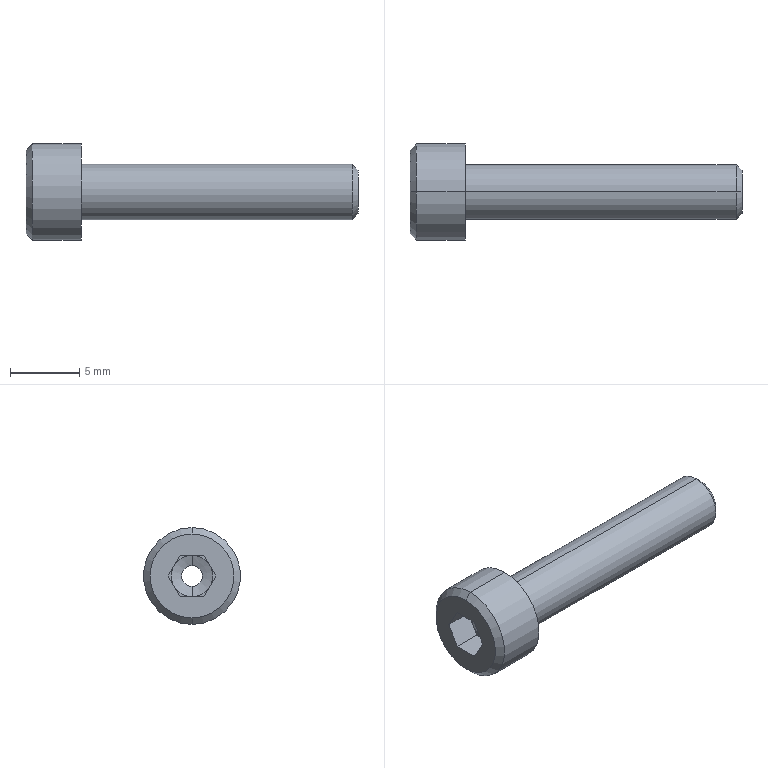Part | SolidWorks | features ICE 1, RevCut 1, Revolution 1 | 1 solid | 27 faces | box 24 x 7 x 7 mm | volume 346.79 mm3 | plane 15 | cylinder 6 | cone 6 | commonest cylinder face diameters 1.5 x2 4 x2 7 x2
STEP:
#1=CARTESIAN_POINT('',(20.,0.,-0.75));
#2=VERTEX_POINT('',#1);
#3=CARTESIAN_POINT('',(20.,0.,0.75));
#4=VERTEX_POINT('',#3);
#5=CARTESIAN_POINT('',(20.,0.,0.));
#6=DIRECTION('',(-1.,0.,0.));
#7=DIRECTION('',(0.,0.,1.));
#8=AXIS2_PLACEMENT_3D('',#5,#6,#7);
#9=CIRCLE('',#8,0.75);
#10=EDGE_CURVE('',#2,#4,#9,.T.);
#11=ORIENTED_EDGE('',*,*,#10,.F.);
#12=CARTESIAN_POINT('',(-1.727,0.,-0.75));
#13=VERTEX_POINT('',#12);
#14=CARTESIAN_POINT('',(20.,0.,-0.75));
#15=DIRECTION('',(-1.,0.,0.));
#16=VECTOR('',#15,1000.);
#17=LINE('',#14,#16);
#18=EDGE_CURVE('',#2,#13,#17,.T.);
#19=ORIENTED_EDGE('',*,*,#18,.T.);
#20=CARTESIAN_POINT('',(-1.727,0.,0.75));
#21=VERTEX_POINT('',#20);
#22=CARTESIAN_POINT('',(-1.727,0.,0.));
#23=DIRECTION('',(-1.,0.,0.));
#24=DIRECTION('',(0.,0.,1.));
#25=AXIS2_PLACEMENT_3D('',#22,#23,#24);
#26=CIRCLE('',#25,0.75);
#27=EDGE_CURVE('',#13,#21,#26,.T.);
#28=ORIENTED_EDGE('',*,*,#27,.T.);
#29=CARTESIAN_POINT('',(20.,0.,0.75));
#30=DIRECTION('',(-1.,0.,0.));
#31=VECTOR('',#30,1000.);
#32=LINE('',#29,#31);
#33=EDGE_CURVE('',#4,#21,#32,.T.);
#34=ORIENTED_EDGE('',*,*,#33,.F.);
#35=EDGE_LOOP('',(#11,#19,#28,#34));
#36=FACE_OUTER_BOUND('',#35,.T.);
#37=CARTESIAN_POINT('',(20.,0.,0.));
#38=DIRECTION('',(-1.,0.,0.));
#39=DIRECTION('',(0.,0.,1.));
#40=AXIS2_PLACEMENT_3D('',#37,#38,#39);
#41=CYLINDRICAL_SURFACE('',#40,0.75);
#42=ADVANCED_FACE('',(#36),#41,.F.);
#43=ORIENTED_EDGE('',*,*,#27,.F.);
#44=CARTESIAN_POINT('',(-2.,0.,-1.5));
#45=VERTEX_POINT('',#44);
#46=CARTESIAN_POINT('',(-1.727,0.,-0.75));
#47=DIRECTION('',(-0.342,0.,-0.9397));
#48=VECTOR('',#47,1000.);
#49=LINE('',#46,#48);
#50=EDGE_CURVE('',#13,#45,#49,.T.);
#51=ORIENTED_EDGE('',*,*,#50,.T.);
#52=CARTESIAN_POINT('',(-2.,-1.299,-0.75));
#53=VERTEX_POINT('',#52);
#54=CARTESIAN_POINT('',(-2.,0.,0.));
#55=DIRECTION('',(-1.,0.,0.));
#56=DIRECTION('',(0.,0.,1.));
#57=AXIS2_PLACEMENT_3D('',#54,#55,#56);
#58=CIRCLE('',#57,1.5);
#59=EDGE_CURVE('',#45,#53,#58,.T.);
#60=ORIENTED_EDGE('',*,*,#59,.T.);
#61=CARTESIAN_POINT('',(-2.,-1.299,0.75));
#62=VERTEX_POINT('',#61);
#63=CARTESIAN_POINT('',(-2.,0.,0.));
#64=DIRECTION('',(-1.,0.,0.));
#65=DIRECTION('',(0.,0.,1.));
#66=AXIS2_PLACEMENT_3D('',#63,#64,#65);
#67=CIRCLE('',#66,1.5);
#68=EDGE_CURVE('',#53,#62,#67,.T.);
#69=ORIENTED_EDGE('',*,*,#68,.T.);
#70=CARTESIAN_POINT('',(-2.,0.,1.5));
#71=VERTEX_POINT('',#70);
#72=CARTESIAN_POINT('',(-2.,0.,0.));
#73=DIRECTION('',(-1.,0.,0.));
#74=DIRECTION('',(0.,0.,1.));
#75=AXIS2_PLACEMENT_3D('',#72,#73,#74);
#76=CIRCLE('',#75,1.5);
#77=EDGE_CURVE('',#62,#71,#76,.T.);
#78=ORIENTED_EDGE('',*,*,#77,.T.);
#79=CARTESIAN_POINT('',(-1.727,0.,0.75));
#80=DIRECTION('',(-0.342,0.,0.9397));
#81=VECTOR('',#80,1000.);
#82=LINE('',#79,#81);
#83=EDGE_CURVE('',#21,#71,#82,.T.);
#84=ORIENTED_EDGE('',*,*,#83,.F.);
#85=EDGE_LOOP('',(#43,#51,#60,#69,#78,#84));
#86=FACE_OUTER_BOUND('',#85,.T.);
#87=CARTESIAN_POINT('',(-1.727,0.,0.));
#88=DIRECTION('',(-1.,0.,0.));
#89=DIRECTION('',(0.,0.,1.));
#90=AXIS2_PLACEMENT_3D('',#87,#88,#89);
#91=CONICAL_SURFACE('',#90,0.75,1.222);
#92=ADVANCED_FACE('',(#86),#91,.F.);
#93=CARTESIAN_POINT('',(20.,0.,1.57));
#94=VERTEX_POINT('',#93);
#95=CARTESIAN_POINT('',(20.,0.,-1.57));
#96=VERTEX_POINT('',#95);
#97=CARTESIAN_POINT('',(20.,0.,0.));
#98=DIRECTION('',(-1.,0.,0.));
#99=DIRECTION('',(0.,0.,1.));
#100=AXIS2_PLACEMENT_3D('',#97,#98,#99);
#101=CIRCLE('',#100,1.57);
#102=EDGE_CURVE('',#94,#96,#101,.T.);
#103=ORIENTED_EDGE('',*,*,#102,.T.);
#104=CARTESIAN_POINT('',(19.57,0.,-2.));
#105=VERTEX_POINT('',#104);
#106=CARTESIAN_POINT('',(20.,0.,-1.57));
#107=DIRECTION('',(-0.7071,0.,-0.7071));
#108=VECTOR('',#107,1000.);
#109=LINE('',#106,#108);
#110=EDGE_CURVE('',#96,#105,#109,.T.);
#111=ORIENTED_EDGE('',*,*,#110,.T.);
#112=CARTESIAN_POINT('',(19.57,0.,2.));
#113=VERTEX_POINT('',#112);
#114=CARTESIAN_POINT('',(19.57,0.,0.));
#115=DIRECTION('',(-1.,0.,0.));
#116=DIRECTION('',(0.,0.,1.));
#117=AXIS2_PLACEMENT_3D('',#114,#115,#116);
#118=CIRCLE('',#117,2.);
#119=EDGE_CURVE('',#113,#105,#118,.T.);
#120=ORIENTED_EDGE('',*,*,#119,.F.);
#121=CARTESIAN_POINT('',(20.,0.,1.57));
#122=DIRECTION('',(-0.7071,0.,0.7071));
#123=VECTOR('',#122,1000.);
#124=LINE('',#121,#123);
#125=EDGE_CURVE('',#94,#113,#124,.T.);
#126=ORIENTED_EDGE('',*,*,#125,.F.);
#127=EDGE_LOOP('',(#103,#111,#120,#126));
#128=FACE_OUTER_BOUND('',#127,.T.);
#129=CARTESIAN_POINT('',(20.,0.,0.));
#130=DIRECTION('',(-1.,0.,0.));
#131=DIRECTION('',(0.,0.,1.));
#132=AXIS2_PLACEMENT_3D('',#129,#130,#131);
#133=CONICAL_SURFACE('',#132,1.57,0.7854);
#134=ADVANCED_FACE('',(#128),#133,.T.);
#135=ORIENTED_EDGE('',*,*,#119,.T.);
#136=CARTESIAN_POINT('',(0.,0.,-2.));
#137=VERTEX_POINT('',#136);
#138=CARTESIAN_POINT('',(20.,0.,-2.));
#139=DIRECTION('',(-1.,0.,0.));
#140=VECTOR('',#139,1000.);
#141=LINE('',#138,#140);
#142=EDGE_CURVE('',#105,#137,#141,.T.);
#143=ORIENTED_EDGE('',*,*,#142,.T.);
#144=CARTESIAN_POINT('',(0.,0.,2.));
#145=VERTEX_POINT('',#144);
#146=CARTESIAN_POINT('',(0.,0.,0.));
#147=DIRECTION('',(-1.,0.,0.));
#148=DIRECTION('',(0.,0.,1.));
#149=AXIS2_PLACEMENT_3D('',#146,#147,#148);
#150=CIRCLE('',#149,2.);
#151=EDGE_CURVE('',#145,#137,#150,.T.);
#152=ORIENTED_EDGE('',*,*,#151,.F.);
#153=CARTESIAN_POINT('',(20.,0.,2.));
#154=DIRECTION('',(-1.,0.,0.));
#155=VECTOR('',#154,1000.);
#156=LINE('',#153,#155);
#157=EDGE_CURVE('',#113,#145,#156,.T.);
#158=ORIENTED_EDGE('',*,*,#157,.F.);
#159=EDGE_LOOP('',(#135,#143,#152,#158));
#160=FACE_OUTER_BOUND('',#159,.T.);
#161=CARTESIAN_POINT('',(20.,0.,0.));
#162=DIRECTION('',(-1.,0.,0.));
#163=DIRECTION('',(0.,0.,1.));
#164=AXIS2_PLACEMENT_3D('',#161,#162,#163);
#165=CYLINDRICAL_SURFACE('',#164,2.);
#166=ADVANCED_FACE('',(#160),#165,.T.);
#167=CARTESIAN_POINT('',(0.,0.,3.5));
#168=VERTEX_POINT('',#167);
#169=CARTESIAN_POINT('',(0.,0.,-3.5));
#170=VERTEX_POINT('',#169);
#171=CARTESIAN_POINT('',(0.,0.,0.));
#172=DIRECTION('',(-1.,0.,0.));
#173=DIRECTION('',(0.,0.,1.));
#174=AXIS2_PLACEMENT_3D('',#171,#172,#173);
#175=CIRCLE('',#174,3.5);
#176=EDGE_CURVE('',#168,#170,#175,.T.);
#177=ORIENTED_EDGE('',*,*,#176,.T.);
#178=CARTESIAN_POINT('',(-3.533,0.,-3.5));
#179=VERTEX_POINT('',#178);
#180=CARTESIAN_POINT('',(20.,0.,-3.5));
#181=DIRECTION('',(-1.,0.,0.));
#182=VECTOR('',#181,1000.);
#183=LINE('',#180,#182);
#184=EDGE_CURVE('',#170,#179,#183,.T.);
#185=ORIENTED_EDGE('',*,*,#184,.T.);
#186=CARTESIAN_POINT('',(-3.533,0.,3.5));
#187=VERTEX_POINT('',#186);
#188=CARTESIAN_POINT('',(-3.533,0.,0.));
#189=DIRECTION('',(-1.,0.,0.));
#190=DIRECTION('',(0.,0.,1.));
#191=AXIS2_PLACEMENT_3D('',#188,#189,#190);
#192=CIRCLE('',#191,3.5);
#193=EDGE_CURVE('',#187,#179,#192,.T.);
#194=ORIENTED_EDGE('',*,*,#193,.F.);
#195=CARTESIAN_POINT('',(20.,0.,3.5));
#196=DIRECTION('',(-1.,0.,0.));
#197=VECTOR('',#196,1000.);
#198=LINE('',#195,#197);
#199=EDGE_CURVE('',#168,#187,#198,.T.);
#200=ORIENTED_EDGE('',*,*,#199,.F.);
#201=EDGE_LOOP('',(#177,#185,#194,#200));
#202=FACE_OUTER_BOUND('',#201,.T.);
#203=CARTESIAN_POINT('',(20.,0.,0.));
#204=DIRECTION('',(-1.,0.,0.));
#205=DIRECTION('',(0.,0.,1.));
#206=AXIS2_PLACEMENT_3D('',#203,#204,#205);
#207=CYLINDRICAL_SURFACE('',#206,3.5);
#208=ADVANCED_FACE('',(#202),#207,.T.);
#209=CARTESIAN_POINT('',(-4.,0.,3.033));
#210=VERTEX_POINT('',#209);
#211=CARTESIAN_POINT('',(-4.,0.,-3.033));
#212=VERTEX_POINT('',#211);
#213=CARTESIAN_POINT('',(-4.,0.,0.));
#214=DIRECTION('',(-1.,0.,0.));
#215=DIRECTION('',(0.,0.,1.));
#216=AXIS2_PLACEMENT_3D('',#213,#214,#215);
#217=CIRCLE('',#216,3.033);
#218=EDGE_CURVE('',#210,#212,#217,.T.);
#219=ORIENTED_EDGE('',*,*,#218,.F.);
#220=CARTESIAN_POINT('',(-3.533,0.,3.5));
#221=DIRECTION('',(0.7071,0.,0.7071));
#222=VECTOR('',#221,1000.);
#223=LINE('',#220,#222);
#224=EDGE_CURVE('',#210,#187,#223,.T.);
#225=ORIENTED_EDGE('',*,*,#224,.T.);
#226=ORIENTED_EDGE('',*,*,#193,.T.);
#227=CARTESIAN_POINT('',(-3.533,0.,-3.5));
#228=DIRECTION('',(0.7071,0.,-0.7071));
#229=VECTOR('',#228,1000.);
#230=LINE('',#227,#229);
#231=EDGE_CURVE('',#212,#179,#230,.T.);
#232=ORIENTED_EDGE('',*,*,#231,.F.);
#233=EDGE_LOOP('',(#219,#225,#226,#232));
#234=FACE_OUTER_BOUND('',#233,.T.);
#235=CARTESIAN_POINT('',(-3.533,0.,0.));
#236=DIRECTION('',(1.,0.,0.));
#237=DIRECTION('',(0.,0.,-1.));
#238=AXIS2_PLACEMENT_3D('',#235,#236,#237);
#239=CONICAL_SURFACE('',#238,3.5,0.7854);
#240=ADVANCED_FACE('',(#234),#239,.T.);
#241=CARTESIAN_POINT('',(-4.,0.,0.));
#242=DIRECTION('',(-1.,0.,0.));
#243=DIRECTION('',(0.,0.,1.));
#244=AXIS2_PLACEMENT_3D('',#241,#242,#243);
#245=CIRCLE('',#244,3.033);
#246=EDGE_CURVE('',#212,#210,#245,.T.);
#247=ORIENTED_EDGE('',*,*,#246,.T.);
#248=ORIENTED_EDGE('',*,*,#218,.T.);
#249=EDGE_LOOP('',(#247,#248));
#250=FACE_OUTER_BOUND('',#249,.T.);
#251=CARTESIAN_POINT('',(-4.,-0.866,1.5));
#252=VERTEX_POINT('',#251);
#253=CARTESIAN_POINT('',(-4.,-1.732,0.));
#254=VERTEX_POINT('',#253);
#255=CARTESIAN_POINT('',(-4.,-0.866,1.5));
#256=DIRECTION('',(0.,-0.5,-0.866));
#257=VECTOR('',#256,1000.);
#258=LINE('',#255,#257);
#259=EDGE_CURVE('',#252,#254,#258,.T.);
#260=ORIENTED_EDGE('',*,*,#259,.T.);
#261=CARTESIAN_POINT('',(-4.,-0.866,-1.5));
#262=VERTEX_POINT('',#261);
#263=CARTESIAN_POINT('',(-4.,-1.732,0.));
#264=DIRECTION('',(0.,0.5,-0.866));
#265=VECTOR('',#264,1000.);
#266=LINE('',#263,#265);
#267=EDGE_CURVE('',#254,#262,#266,.T.);
#268=ORIENTED_EDGE('',*,*,#267,.T.);
#269=CARTESIAN_POINT('',(-4.,0.866,-1.5));
#270=VERTEX_POINT('',#269);
#271=CARTESIAN_POINT('',(-4.,-0.866,-1.5));
#272=DIRECTION('',(0.,1.,0.));
#273=VECTOR('',#272,1000.);
#274=LINE('',#271,#273);
#275=EDGE_CURVE('',#262,#270,#274,.T.);
#276=ORIENTED_EDGE('',*,*,#275,.T.);
#277=CARTESIAN_POINT('',(-4.,1.732,0.));
#278=VERTEX_POINT('',#277);
#279=CARTESIAN_POINT('',(-4.,0.866,-1.5));
#280=DIRECTION('',(0.,0.5,0.866));
#281=VECTOR('',#280,1000.);
#282=LINE('',#279,#281);
#283=EDGE_CURVE('',#270,#278,#282,.T.);
#284=ORIENTED_EDGE('',*,*,#283,.T.);
#285=CARTESIAN_POINT('',(-4.,0.866,1.5));
#286=VERTEX_POINT('',#285);
#287=CARTESIAN_POINT('',(-4.,1.732,0.));
#288=DIRECTION('',(0.,-0.5,0.866));
#289=VECTOR('',#288,1000.);
#290=LINE('',#287,#289);
#291=EDGE_CURVE('',#278,#286,#290,.T.);
#292=ORIENTED_EDGE('',*,*,#291,.T.);
#293=CARTESIAN_POINT('',(-4.,0.866,1.5));
#294=DIRECTION('',(0.,-1.,0.));
#295=VECTOR('',#294,1000.);
#296=LINE('',#293,#295);
#297=EDGE_CURVE('',#286,#252,#296,.T.);
#298=ORIENTED_EDGE('',*,*,#297,.T.);
#299=EDGE_LOOP('',(#260,#268,#276,#284,#292,#298));
#300=FACE_BOUND('',#299,.T.);
#301=CARTESIAN_POINT('',(-4.,0.,0.));
#302=DIRECTION('',(1.,0.,0.));
#303=DIRECTION('',(0.,0.,-1.));
#304=AXIS2_PLACEMENT_3D('',#301,#302,#303);
#305=PLANE('',#304);
#306=ADVANCED_FACE('',(#250,#300),#305,.F.);
#307=ORIENTED_EDGE('',*,*,#102,.F.);
#308=CARTESIAN_POINT('',(20.,0.,0.));
#309=DIRECTION('',(-1.,0.,0.));
#310=DIRECTION('',(0.,0.,1.));
#311=AXIS2_PLACEMENT_3D('',#308,#309,#310);
#312=CIRCLE('',#311,1.57);
#313=EDGE_CURVE('',#96,#94,#312,.T.);
#314=ORIENTED_EDGE('',*,*,#313,.F.);
#315=EDGE_LOOP('',(#307,#314));
#316=FACE_OUTER_BOUND('',#315,.T.);
#317=CARTESIAN_POINT('',(20.,0.,0.));
#318=DIRECTION('',(-1.,0.,0.));
#319=DIRECTION('',(0.,0.,1.));
#320=AXIS2_PLACEMENT_3D('',#317,#318,#319);
#321=CIRCLE('',#320,0.75);
#322=EDGE_CURVE('',#4,#2,#321,.T.);
#323=ORIENTED_EDGE('',*,*,#322,.T.);
#324=ORIENTED_EDGE('',*,*,#10,.T.);
#325=EDGE_LOOP('',(#323,#324));
#326=FACE_BOUND('',#325,.T.);
#327=CARTESIAN_POINT('',(20.,1.57,0.));
#328=DIRECTION('',(-1.,0.,0.));
#329=DIRECTION('',(0.,0.,1.));
#330=AXIS2_PLACEMENT_3D('',#327,#328,#329);
#331=PLANE('',#330);
#332=ADVANCED_FACE('',(#316,#326),#331,.F.);
#333=ORIENTED_EDGE('',*,*,#224,.F.);
#334=ORIENTED_EDGE('',*,*,#246,.F.);
#335=ORIENTED_EDGE('',*,*,#231,.T.);
#336=CARTESIAN_POINT('',(-3.533,0.,0.));
#337=DIRECTION('',(-1.,0.,0.));
#338=DIRECTION('',(0.,0.,1.));
#339=AXIS2_PLACEMENT_3D('',#336,#337,#338);
#340=CIRCLE('',#339,3.5);
#341=EDGE_CURVE('',#179,#187,#340,.T.);
#342=ORIENTED_EDGE('',*,*,#341,.T.);
#343=EDGE_LOOP('',(#333,#334,#335,#342));
#344=FACE_OUTER_BOUND('',#343,.T.);
#345=CARTESIAN_POINT('',(-3.533,0.,0.));
#346=DIRECTION('',(1.,0.,0.));
#347=DIRECTION('',(0.,0.,-1.));
#348=AXIS2_PLACEMENT_3D('',#345,#346,#347);
#349=CONICAL_SURFACE('',#348,3.5,0.7854);
#350=ADVANCED_FACE('',(#344),#349,.T.);
#351=ORIENTED_EDGE('',*,*,#184,.F.);
#352=CARTESIAN_POINT('',(0.,0.,0.));
#353=DIRECTION('',(-1.,0.,0.));
#354=DIRECTION('',(0.,0.,1.));
#355=AXIS2_PLACEMENT_3D('',#352,#353,#354);
#356=CIRCLE('',#355,3.5);
#357=EDGE_CURVE('',#170,#168,#356,.T.);
#358=ORIENTED_EDGE('',*,*,#357,.T.);
#359=ORIENTED_EDGE('',*,*,#199,.T.);
#360=ORIENTED_EDGE('',*,*,#341,.F.);
#361=EDGE_LOOP('',(#351,#358,#359,#360));
#362=FACE_OUTER_BOUND('',#361,.T.);
#363=CARTESIAN_POINT('',(20.,0.,0.));
#364=DIRECTION('',(-1.,0.,0.));
#365=DIRECTION('',(0.,0.,1.));
#366=AXIS2_PLACEMENT_3D('',#363,#364,#365);
#367=CYLINDRICAL_SURFACE('',#366,3.5);
#368=ADVANCED_FACE('',(#362),#367,.T.);
#369=ORIENTED_EDGE('',*,*,#176,.F.);
#370=ORIENTED_EDGE('',*,*,#357,.F.);
#371=EDGE_LOOP('',(#369,#370));
#372=FACE_OUTER_BOUND('',#371,.T.);
#373=ORIENTED_EDGE('',*,*,#151,.T.);
#374=CARTESIAN_POINT('',(0.,0.,0.));
#375=DIRECTION('',(-1.,0.,0.));
#376=DIRECTION('',(0.,0.,1.));
#377=AXIS2_PLACEMENT_3D('',#374,#375,#376);
#378=CIRCLE('',#377,2.);
#379=EDGE_CURVE('',#137,#145,#378,.T.);
#380=ORIENTED_EDGE('',*,*,#379,.T.);
#381=EDGE_LOOP('',(#373,#380));
#382=FACE_BOUND('',#381,.T.);
#383=CARTESIAN_POINT('',(0.,3.5,0.));
#384=DIRECTION('',(-1.,0.,0.));
#385=DIRECTION('',(0.,0.,1.));
#386=AXIS2_PLACEMENT_3D('',#383,#384,#385);
#387=PLANE('',#386);
#388=ADVANCED_FACE('',(#372,#382),#387,.F.);
#389=ORIENTED_EDGE('',*,*,#142,.F.);
#390=CARTESIAN_POINT('',(19.57,0.,0.));
#391=DIRECTION('',(-1.,0.,0.));
#392=DIRECTION('',(0.,0.,1.));
#393=AXIS2_PLACEMENT_3D('',#390,#391,#392);
#394=CIRCLE('',#393,2.);
#395=EDGE_CURVE('',#105,#113,#394,.T.);
#396=ORIENTED_EDGE('',*,*,#395,.T.);
#397=ORIENTED_EDGE('',*,*,#157,.T.);
#398=ORIENTED_EDGE('',*,*,#379,.F.);
#399=EDGE_LOOP('',(#389,#396,#397,#398));
#400=FACE_OUTER_BOUND('',#399,.T.);
#401=CARTESIAN_POINT('',(20.,0.,0.));
#402=DIRECTION('',(-1.,0.,0.));
#403=DIRECTION('',(0.,0.,1.));
#404=AXIS2_PLACEMENT_3D('',#401,#402,#403);
#405=CYLINDRICAL_SURFACE('',#404,2.);
#406=ADVANCED_FACE('',(#400),#405,.T.);
#407=ORIENTED_EDGE('',*,*,#110,.F.);
#408=ORIENTED_EDGE('',*,*,#313,.T.);
#409=ORIENTED_EDGE('',*,*,#125,.T.);
#410=ORIENTED_EDGE('',*,*,#395,.F.);
#411=EDGE_LOOP('',(#407,#408,#409,#410));
#412=FACE_OUTER_BOUND('',#411,.T.);
#413=CARTESIAN_POINT('',(20.,0.,0.));
#414=DIRECTION('',(-1.,0.,0.));
#415=DIRECTION('',(0.,0.,1.));
#416=AXIS2_PLACEMENT_3D('',#413,#414,#415);
#417=CONICAL_SURFACE('',#416,1.57,0.7854);
#418=ADVANCED_FACE('',(#412),#417,.T.);
#419=ORIENTED_EDGE('',*,*,#50,.F.);
#420=CARTESIAN_POINT('',(-1.727,0.,0.));
#421=DIRECTION('',(-1.,0.,0.));
#422=DIRECTION('',(0.,0.,1.));
#423=AXIS2_PLACEMENT_3D('',#420,#421,#422);
#424=CIRCLE('',#423,0.75);
#425=EDGE_CURVE('',#21,#13,#424,.T.);
#426=ORIENTED_EDGE('',*,*,#425,.F.);
#427=ORIENTED_EDGE('',*,*,#83,.T.);
#428=CARTESIAN_POINT('',(-2.,1.299,0.75));
#429=VERTEX_POINT('',#428);
#430=CARTESIAN_POINT('',(-2.,0.,0.));
#431=DIRECTION('',(-1.,0.,0.));
#432=DIRECTION('',(0.,0.,1.));
#433=AXIS2_PLACEMENT_3D('',#430,#431,#432);
#434=CIRCLE('',#433,1.5);
#435=EDGE_CURVE('',#71,#429,#434,.T.);
#436=ORIENTED_EDGE('',*,*,#435,.T.);
#437=CARTESIAN_POINT('',(-2.,1.299,-0.75));
#438=VERTEX_POINT('',#437);
#439=CARTESIAN_POINT('',(-2.,0.,0.));
#440=DIRECTION('',(-1.,0.,0.));
#441=DIRECTION('',(0.,0.,1.));
#442=AXIS2_PLACEMENT_3D('',#439,#440,#441);
#443=CIRCLE('',#442,1.5);
#444=EDGE_CURVE('',#429,#438,#443,.T.);
#445=ORIENTED_EDGE('',*,*,#444,.T.);
#446=CARTESIAN_POINT('',(-2.,0.,0.));
#447=DIRECTION('',(-1.,0.,0.));
#448=DIRECTION('',(0.,0.,1.));
#449=AXIS2_PLACEMENT_3D('',#446,#447,#448);
#450=CIRCLE('',#449,1.5);
#451=EDGE_CURVE('',#438,#45,#450,.T.);
#452=ORIENTED_EDGE('',*,*,#451,.T.);
#453=EDGE_LOOP('',(#419,#426,#427,#436,#445,#452));
#454=FACE_OUTER_BOUND('',#453,.T.);
#455=CARTESIAN_POINT('',(-1.727,0.,0.));
#456=DIRECTION('',(-1.,0.,0.));
#457=DIRECTION('',(0.,0.,1.));
#458=AXIS2_PLACEMENT_3D('',#455,#456,#457);
#459=CONICAL_SURFACE('',#458,0.75,1.222);
#460=ADVANCED_FACE('',(#454),#459,.F.);
#461=ORIENTED_EDGE('',*,*,#18,.F.);
#462=ORIENTED_EDGE('',*,*,#322,.F.);
#463=ORIENTED_EDGE('',*,*,#33,.T.);
#464=ORIENTED_EDGE('',*,*,#425,.T.);
#465=EDGE_LOOP('',(#461,#462,#463,#464));
#466=FACE_OUTER_BOUND('',#465,.T.);
#467=CARTESIAN_POINT('',(20.,0.,0.));
#468=DIRECTION('',(-1.,0.,0.));
#469=DIRECTION('',(0.,0.,1.));
#470=AXIS2_PLACEMENT_3D('',#467,#468,#469);
#471=CYLINDRICAL_SURFACE('',#470,0.75);
#472=ADVANCED_FACE('',(#466),#471,.F.);
#473=CARTESIAN_POINT('',(-2.,1.732,0.));
#474=VERTEX_POINT('',#473);
#475=CARTESIAN_POINT('',(-2.,1.732,0.));
#476=DIRECTION('',(0.,-0.5,0.866));
#477=VECTOR('',#476,1000.);
#478=LINE('',#475,#477);
#479=EDGE_CURVE('',#474,#429,#478,.T.);
#480=ORIENTED_EDGE('',*,*,#479,.T.);
#481=CARTESIAN_POINT('',(-2.,0.866,1.5));
#482=VERTEX_POINT('',#481);
#483=CARTESIAN_POINT('',(-2.,1.732,0.));
#484=DIRECTION('',(0.,-0.5,0.866));
#485=VECTOR('',#484,1000.);
#486=LINE('',#483,#485);
#487=EDGE_CURVE('',#429,#482,#486,.T.);
#488=ORIENTED_EDGE('',*,*,#487,.T.);
#489=CARTESIAN_POINT('',(-2.,0.866,1.5));
#490=DIRECTION('',(-1.,0.,0.));
#491=VECTOR('',#490,1000.);
#492=LINE('',#489,#491);
#493=EDGE_CURVE('',#482,#286,#492,.T.);
#494=ORIENTED_EDGE('',*,*,#493,.T.);
#495=ORIENTED_EDGE('',*,*,#291,.F.);
#496=CARTESIAN_POINT('',(-2.,1.732,0.));
#497=DIRECTION('',(-1.,0.,0.));
#498=VECTOR('',#497,1000.);
#499=LINE('',#496,#498);
#500=EDGE_CURVE('',#474,#278,#499,.T.);
#501=ORIENTED_EDGE('',*,*,#500,.F.);
#502=EDGE_LOOP('',(#480,#488,#494,#495,#501));
#503=FACE_OUTER_BOUND('',#502,.T.);
#504=CARTESIAN_POINT('',(-2.,1.732,0.));
#505=DIRECTION('',(0.,-0.866,-0.5));
#506=DIRECTION('',(0.,0.5,-0.866));
#507=AXIS2_PLACEMENT_3D('',#504,#505,#506);
#508=PLANE('',#507);
#509=ADVANCED_FACE('',(#503),#508,.T.);
#510=CARTESIAN_POINT('',(-2.,0.866,1.5));
#511=DIRECTION('',(0.,-1.,0.));
#512=VECTOR('',#511,1000.);
#513=LINE('',#510,#512);
#514=EDGE_CURVE('',#482,#71,#513,.T.);
#515=ORIENTED_EDGE('',*,*,#514,.T.);
#516=CARTESIAN_POINT('',(-2.,-0.866,1.5));
#517=VERTEX_POINT('',#516);
#518=CARTESIAN_POINT('',(-2.,0.866,1.5));
#519=DIRECTION('',(0.,-1.,0.));
#520=VECTOR('',#519,1000.);
#521=LINE('',#518,#520);
#522=EDGE_CURVE('',#71,#517,#521,.T.);
#523=ORIENTED_EDGE('',*,*,#522,.T.);
#524=CARTESIAN_POINT('',(-2.,-0.866,1.5));
#525=DIRECTION('',(-1.,0.,0.));
#526=VECTOR('',#525,1000.);
#527=LINE('',#524,#526);
#528=EDGE_CURVE('',#517,#252,#527,.T.);
#529=ORIENTED_EDGE('',*,*,#528,.T.);
#530=ORIENTED_EDGE('',*,*,#297,.F.);
#531=ORIENTED_EDGE('',*,*,#493,.F.);
#532=EDGE_LOOP('',(#515,#523,#529,#530,#531));
#533=FACE_OUTER_BOUND('',#532,.T.);
#534=CARTESIAN_POINT('',(-2.,0.866,1.5));
#535=DIRECTION('',(0.,0.,-1.));
#536=DIRECTION('',(-1.,0.,0.));
#537=AXIS2_PLACEMENT_3D('',#534,#535,#536);
#538=PLANE('',#537);
#539=ADVANCED_FACE('',(#533),#538,.T.);
#540=CARTESIAN_POINT('',(-2.,-0.866,1.5));
#541=DIRECTION('',(0.,-0.5,-0.866));
#542=VECTOR('',#541,1000.);
#543=LINE('',#540,#542);
#544=EDGE_CURVE('',#517,#62,#543,.T.);
#545=ORIENTED_EDGE('',*,*,#544,.T.);
#546=CARTESIAN_POINT('',(-2.,-1.732,0.));
#547=VERTEX_POINT('',#546);
#548=CARTESIAN_POINT('',(-2.,-0.866,1.5));
#549=DIRECTION('',(0.,-0.5,-0.866));
#550=VECTOR('',#549,1000.);
#551=LINE('',#548,#550);
#552=EDGE_CURVE('',#62,#547,#551,.T.);
#553=ORIENTED_EDGE('',*,*,#552,.T.);
#554=CARTESIAN_POINT('',(-2.,-1.732,0.));
#555=DIRECTION('',(-1.,0.,0.));
#556=VECTOR('',#555,1000.);
#557=LINE('',#554,#556);
#558=EDGE_CURVE('',#547,#254,#557,.T.);
#559=ORIENTED_EDGE('',*,*,#558,.T.);
#560=ORIENTED_EDGE('',*,*,#259,.F.);
#561=ORIENTED_EDGE('',*,*,#528,.F.);
#562=EDGE_LOOP('',(#545,#553,#559,#560,#561));
#563=FACE_OUTER_BOUND('',#562,.T.);
#564=CARTESIAN_POINT('',(-2.,-0.866,1.5));
#565=DIRECTION('',(0.,0.866,-0.5));
#566=DIRECTION('',(0.,0.5,0.866));
#567=AXIS2_PLACEMENT_3D('',#564,#565,#566);
#568=PLANE('',#567);
#569=ADVANCED_FACE('',(#563),#568,.T.);
#570=CARTESIAN_POINT('',(-2.,-1.732,0.));
#571=DIRECTION('',(0.,0.5,-0.866));
#572=VECTOR('',#571,1000.);
#573=LINE('',#570,#572);
#574=EDGE_CURVE('',#547,#53,#573,.T.);
#575=ORIENTED_EDGE('',*,*,#574,.T.);
#576=CARTESIAN_POINT('',(-2.,-0.866,-1.5));
#577=VERTEX_POINT('',#576);
#578=CARTESIAN_POINT('',(-2.,-1.732,0.));
#579=DIRECTION('',(0.,0.5,-0.866));
#580=VECTOR('',#579,1000.);
#581=LINE('',#578,#580);
#582=EDGE_CURVE('',#53,#577,#581,.T.);
#583=ORIENTED_EDGE('',*,*,#582,.T.);
#584=CARTESIAN_POINT('',(-2.,-0.866,-1.5));
#585=DIRECTION('',(-1.,0.,0.));
#586=VECTOR('',#585,1000.);
#587=LINE('',#584,#586);
#588=EDGE_CURVE('',#577,#262,#587,.T.);
#589=ORIENTED_EDGE('',*,*,#588,.T.);
#590=ORIENTED_EDGE('',*,*,#267,.F.);
#591=ORIENTED_EDGE('',*,*,#558,.F.);
#592=EDGE_LOOP('',(#575,#583,#589,#590,#591));
#593=FACE_OUTER_BOUND('',#592,.T.);
#594=CARTESIAN_POINT('',(-2.,-1.732,0.));
#595=DIRECTION('',(0.,0.866,0.5));
#596=DIRECTION('',(0.,-0.5,0.866));
#597=AXIS2_PLACEMENT_3D('',#594,#595,#596);
#598=PLANE('',#597);
#599=ADVANCED_FACE('',(#593),#598,.T.);
#600=CARTESIAN_POINT('',(-2.,-0.866,-1.5));
#601=DIRECTION('',(0.,1.,0.));
#602=VECTOR('',#601,1000.);
#603=LINE('',#600,#602);
#604=EDGE_CURVE('',#577,#45,#603,.T.);
#605=ORIENTED_EDGE('',*,*,#604,.T.);
#606=CARTESIAN_POINT('',(-2.,0.866,-1.5));
#607=VERTEX_POINT('',#606);
#608=CARTESIAN_POINT('',(-2.,-0.866,-1.5));
#609=DIRECTION('',(0.,1.,0.));
#610=VECTOR('',#609,1000.);
#611=LINE('',#608,#610);
#612=EDGE_CURVE('',#45,#607,#611,.T.);
#613=ORIENTED_EDGE('',*,*,#612,.T.);
#614=CARTESIAN_POINT('',(-2.,0.866,-1.5));
#615=DIRECTION('',(-1.,0.,0.));
#616=VECTOR('',#615,1000.);
#617=LINE('',#614,#616);
#618=EDGE_CURVE('',#607,#270,#617,.T.);
#619=ORIENTED_EDGE('',*,*,#618,.T.);
#620=ORIENTED_EDGE('',*,*,#275,.F.);
#621=ORIENTED_EDGE('',*,*,#588,.F.);
#622=EDGE_LOOP('',(#605,#613,#619,#620,#621));
#623=FACE_OUTER_BOUND('',#622,.T.);
#624=CARTESIAN_POINT('',(-2.,-0.866,-1.5));
#625=DIRECTION('',(0.,0.,1.));
#626=DIRECTION('',(1.,0.,0.));
#627=AXIS2_PLACEMENT_3D('',#624,#625,#626);
#628=PLANE('',#627);
#629=ADVANCED_FACE('',(#623),#628,.T.);
#630=CARTESIAN_POINT('',(-2.,0.866,-1.5));
#631=DIRECTION('',(0.,0.5,0.866));
#632=VECTOR('',#631,1000.);
#633=LINE('',#630,#632);
#634=EDGE_CURVE('',#607,#438,#633,.T.);
#635=ORIENTED_EDGE('',*,*,#634,.T.);
#636=CARTESIAN_POINT('',(-2.,0.866,-1.5));
#637=DIRECTION('',(0.,0.5,0.866));
#638=VECTOR('',#637,1000.);
#639=LINE('',#636,#638);
#640=EDGE_CURVE('',#438,#474,#639,.T.);
#641=ORIENTED_EDGE('',*,*,#640,.T.);
#642=ORIENTED_EDGE('',*,*,#500,.T.);
#643=ORIENTED_EDGE('',*,*,#283,.F.);
#644=ORIENTED_EDGE('',*,*,#618,.F.);
#645=EDGE_LOOP('',(#635,#641,#642,#643,#644));
#646=FACE_OUTER_BOUND('',#645,.T.);
#647=CARTESIAN_POINT('',(-2.,0.866,-1.5));
#648=DIRECTION('',(0.,-0.866,0.5));
#649=DIRECTION('',(0.,-0.5,-0.866));
#650=AXIS2_PLACEMENT_3D('',#647,#648,#649);
#651=PLANE('',#650);
#652=ADVANCED_FACE('',(#646),#651,.T.);
#653=ORIENTED_EDGE('',*,*,#451,.F.);
#654=ORIENTED_EDGE('',*,*,#634,.F.);
#655=ORIENTED_EDGE('',*,*,#612,.F.);
#656=EDGE_LOOP('',(#653,#654,#655));
#657=FACE_OUTER_BOUND('',#656,.T.);
#658=CARTESIAN_POINT('',(-2.,0.,0.));
#659=DIRECTION('',(1.,0.,0.));
#660=DIRECTION('',(0.,0.,-1.));
#661=AXIS2_PLACEMENT_3D('',#658,#659,#660);
#662=PLANE('',#661);
#663=ADVANCED_FACE('',(#657),#662,.F.);
#664=ORIENTED_EDGE('',*,*,#444,.F.);
#665=ORIENTED_EDGE('',*,*,#479,.F.);
#666=ORIENTED_EDGE('',*,*,#640,.F.);
#667=EDGE_LOOP('',(#664,#665,#666));
#668=FACE_OUTER_BOUND('',#667,.T.);
#669=CARTESIAN_POINT('',(-2.,0.,0.));
#670=DIRECTION('',(1.,0.,0.));
#671=DIRECTION('',(0.,0.,-1.));
#672=AXIS2_PLACEMENT_3D('',#669,#670,#671);
#673=PLANE('',#672);
#674=ADVANCED_FACE('',(#668),#673,.F.);
#675=ORIENTED_EDGE('',*,*,#435,.F.);
#676=ORIENTED_EDGE('',*,*,#514,.F.);
#677=ORIENTED_EDGE('',*,*,#487,.F.);
#678=EDGE_LOOP('',(#675,#676,#677));
#679=FACE_OUTER_BOUND('',#678,.T.);
#680=CARTESIAN_POINT('',(-2.,0.,0.));
#681=DIRECTION('',(1.,0.,0.));
#682=DIRECTION('',(0.,0.,-1.));
#683=AXIS2_PLACEMENT_3D('',#680,#681,#682);
#684=PLANE('',#683);
#685=ADVANCED_FACE('',(#679),#684,.F.);
#686=ORIENTED_EDGE('',*,*,#77,.F.);
#687=ORIENTED_EDGE('',*,*,#544,.F.);
#688=ORIENTED_EDGE('',*,*,#522,.F.);
#689=EDGE_LOOP('',(#686,#687,#688));
#690=FACE_OUTER_BOUND('',#689,.T.);
#691=CARTESIAN_POINT('',(-2.,0.,0.));
#692=DIRECTION('',(1.,0.,0.));
#693=DIRECTION('',(0.,0.,-1.));
#694=AXIS2_PLACEMENT_3D('',#691,#692,#693);
#695=PLANE('',#694);
#696=ADVANCED_FACE('',(#690),#695,.F.);
#697=ORIENTED_EDGE('',*,*,#68,.F.);
#698=ORIENTED_EDGE('',*,*,#574,.F.);
#699=ORIENTED_EDGE('',*,*,#552,.F.);
#700=EDGE_LOOP('',(#697,#698,#699));
#701=FACE_OUTER_BOUND('',#700,.T.);
#702=CARTESIAN_POINT('',(-2.,0.,0.));
#703=DIRECTION('',(1.,0.,0.));
#704=DIRECTION('',(0.,0.,-1.));
#705=AXIS2_PLACEMENT_3D('',#702,#703,#704);
#706=PLANE('',#705);
#707=ADVANCED_FACE('',(#701),#706,.F.);
#708=ORIENTED_EDGE('',*,*,#59,.F.);
#709=ORIENTED_EDGE('',*,*,#604,.F.);
#710=ORIENTED_EDGE('',*,*,#582,.F.);
#711=EDGE_LOOP('',(#708,#709,#710));
#712=FACE_OUTER_BOUND('',#711,.T.);
#713=CARTESIAN_POINT('',(-2.,0.,0.));
#714=DIRECTION('',(1.,0.,0.));
#715=DIRECTION('',(0.,0.,-1.));
#716=AXIS2_PLACEMENT_3D('',#713,#714,#715);
#717=PLANE('',#716);
#718=ADVANCED_FACE('',(#712),#717,.F.);
#719=CLOSED_SHELL('',(#42,#92,#134,#166,#208,#240,#306,#332,#350,#368,#388,#406,#418,#460,#472,#509,#539,#569,#599,#629,#652,#663,#674,#685,#696,#707,#718));
#720=MANIFOLD_SOLID_BREP('',#719);
#721=CARTESIAN_POINT('',(0.,0.,0.));
#722=DIRECTION('',(0.,0.,1.));
#723=DIRECTION('',(1.,0.,0.));
#724=AXIS2_PLACEMENT_3D('',#721,#722,#723);
#725=(LENGTH_UNIT()NAMED_UNIT(*)SI_UNIT(.MILLI.,.METRE.));
#726=UNCERTAINTY_MEASURE_WITH_UNIT(LENGTH_MEASURE(0.00001),#725,'','');
#727=(NAMED_UNIT(*)PLANE_ANGLE_UNIT()SI_UNIT($,.RADIAN.));
#728=(NAMED_UNIT(*)SI_UNIT($,.STERADIAN.)SOLID_ANGLE_UNIT());
#729=(GEOMETRIC_REPRESENTATION_CONTEXT(3)GLOBAL_UNCERTAINTY_ASSIGNED_CONTEXT((#726))GLOBAL_UNIT_ASSIGNED_CONTEXT((#725,#727,#728))REPRESENTATION_CONTEXT('',''));
#730=ADVANCED_BREP_SHAPE_REPRESENTATION('',(#720,#724),#729);